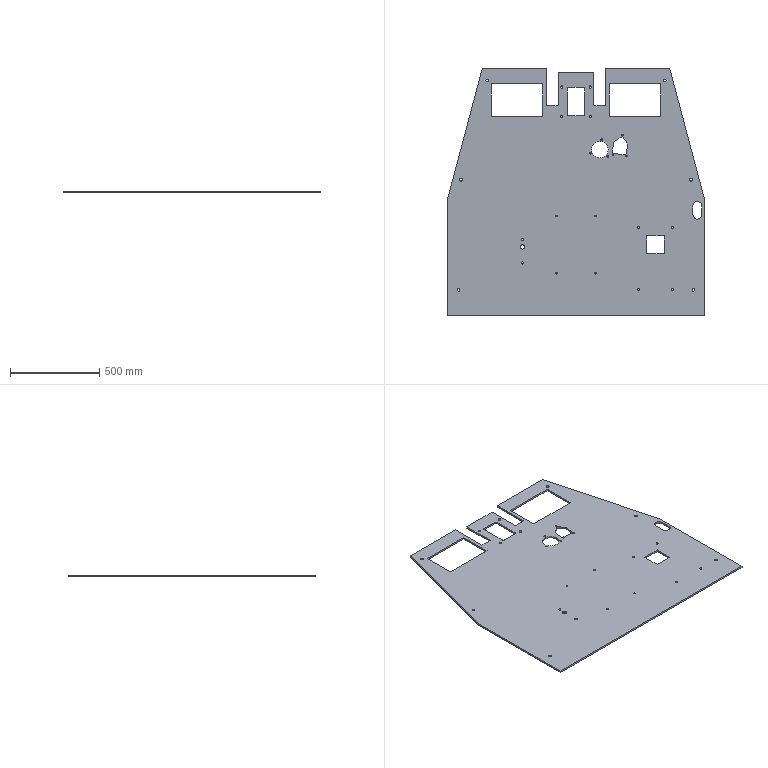Part | SolidWorks | features ICE 21, LPattern 10, Extrusion 1, Fillet 1 | 1 solid | 101 faces | box 1440 x 1385 x 10 mm | volume 16649472 mm3 | cylinder 62 | plane 39 | commonest cylinder face diameters 10 x14 12 x12 16 x12 14 x8 8 x6 20 x4